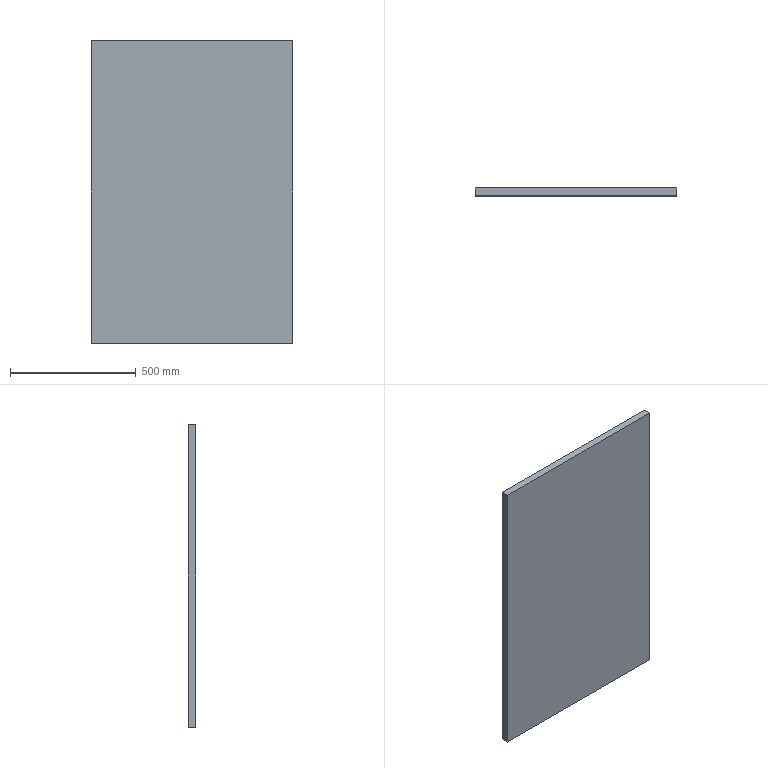Part | 1 solid | 6 faces | box 800 x 30 x 1200 mm | volume 28800000 mm3 | plane 6
STEP:
#1=CARTESIAN_POINT('',(400.,0.,600.));
#2=VERTEX_POINT('',#1);
#3=CARTESIAN_POINT('',(400.,0.,-600.));
#4=VERTEX_POINT('',#3);
#5=CARTESIAN_POINT('',(400.,0.,600.));
#6=DIRECTION('',(0.,0.,-1.));
#7=VECTOR('',#6,1000.);
#8=LINE('',#5,#7);
#9=EDGE_CURVE('',#2,#4,#8,.T.);
#10=ORIENTED_EDGE('',*,*,#9,.T.);
#11=CARTESIAN_POINT('',(400.,30.,-600.));
#12=VERTEX_POINT('',#11);
#13=CARTESIAN_POINT('',(400.,30.,-600.));
#14=DIRECTION('',(0.,-1.,0.));
#15=VECTOR('',#14,1000.);
#16=LINE('',#13,#15);
#17=EDGE_CURVE('',#12,#4,#16,.T.);
#18=ORIENTED_EDGE('',*,*,#17,.F.);
#19=CARTESIAN_POINT('',(400.,30.,600.));
#20=VERTEX_POINT('',#19);
#21=CARTESIAN_POINT('',(400.,30.,600.));
#22=DIRECTION('',(0.,0.,-1.));
#23=VECTOR('',#22,1000.);
#24=LINE('',#21,#23);
#25=EDGE_CURVE('',#20,#12,#24,.T.);
#26=ORIENTED_EDGE('',*,*,#25,.F.);
#27=CARTESIAN_POINT('',(400.,30.,600.));
#28=DIRECTION('',(0.,-1.,0.));
#29=VECTOR('',#28,1000.);
#30=LINE('',#27,#29);
#31=EDGE_CURVE('',#20,#2,#30,.T.);
#32=ORIENTED_EDGE('',*,*,#31,.T.);
#33=EDGE_LOOP('',(#10,#18,#26,#32));
#34=FACE_OUTER_BOUND('',#33,.T.);
#35=CARTESIAN_POINT('',(400.,30.,600.));
#36=DIRECTION('',(-1.,0.,0.));
#37=DIRECTION('',(0.,0.,1.));
#38=AXIS2_PLACEMENT_3D('',#35,#36,#37);
#39=PLANE('',#38);
#40=ADVANCED_FACE('',(#34),#39,.F.);
#41=CARTESIAN_POINT('',(-400.,0.,-600.));
#42=VERTEX_POINT('',#41);
#43=CARTESIAN_POINT('',(-400.,0.,-600.));
#44=DIRECTION('',(-1.,0.,0.));
#45=VECTOR('',#44,1000.);
#46=LINE('',#43,#45);
#47=EDGE_CURVE('',#4,#42,#46,.T.);
#48=ORIENTED_EDGE('',*,*,#47,.T.);
#49=CARTESIAN_POINT('',(-400.,30.,-600.));
#50=VERTEX_POINT('',#49);
#51=CARTESIAN_POINT('',(-400.,30.,-600.));
#52=DIRECTION('',(0.,-1.,0.));
#53=VECTOR('',#52,1000.);
#54=LINE('',#51,#53);
#55=EDGE_CURVE('',#50,#42,#54,.T.);
#56=ORIENTED_EDGE('',*,*,#55,.F.);
#57=CARTESIAN_POINT('',(-400.,30.,-600.));
#58=DIRECTION('',(-1.,0.,0.));
#59=VECTOR('',#58,1000.);
#60=LINE('',#57,#59);
#61=EDGE_CURVE('',#12,#50,#60,.T.);
#62=ORIENTED_EDGE('',*,*,#61,.F.);
#63=ORIENTED_EDGE('',*,*,#17,.T.);
#64=EDGE_LOOP('',(#48,#56,#62,#63));
#65=FACE_OUTER_BOUND('',#64,.T.);
#66=CARTESIAN_POINT('',(-400.,30.,-600.));
#67=DIRECTION('',(0.,0.,1.));
#68=DIRECTION('',(1.,0.,0.));
#69=AXIS2_PLACEMENT_3D('',#66,#67,#68);
#70=PLANE('',#69);
#71=ADVANCED_FACE('',(#65),#70,.F.);
#72=CARTESIAN_POINT('',(-400.,0.,600.));
#73=VERTEX_POINT('',#72);
#74=CARTESIAN_POINT('',(-400.,0.,600.));
#75=DIRECTION('',(0.,0.,1.));
#76=VECTOR('',#75,1000.);
#77=LINE('',#74,#76);
#78=EDGE_CURVE('',#42,#73,#77,.T.);
#79=ORIENTED_EDGE('',*,*,#78,.T.);
#80=CARTESIAN_POINT('',(-400.,30.,600.));
#81=VERTEX_POINT('',#80);
#82=CARTESIAN_POINT('',(-400.,30.,600.));
#83=DIRECTION('',(0.,-1.,0.));
#84=VECTOR('',#83,1000.);
#85=LINE('',#82,#84);
#86=EDGE_CURVE('',#81,#73,#85,.T.);
#87=ORIENTED_EDGE('',*,*,#86,.F.);
#88=CARTESIAN_POINT('',(-400.,30.,600.));
#89=DIRECTION('',(0.,0.,1.));
#90=VECTOR('',#89,1000.);
#91=LINE('',#88,#90);
#92=EDGE_CURVE('',#50,#81,#91,.T.);
#93=ORIENTED_EDGE('',*,*,#92,.F.);
#94=ORIENTED_EDGE('',*,*,#55,.T.);
#95=EDGE_LOOP('',(#79,#87,#93,#94));
#96=FACE_OUTER_BOUND('',#95,.T.);
#97=CARTESIAN_POINT('',(-400.,30.,600.));
#98=DIRECTION('',(1.,0.,0.));
#99=DIRECTION('',(0.,0.,-1.));
#100=AXIS2_PLACEMENT_3D('',#97,#98,#99);
#101=PLANE('',#100);
#102=ADVANCED_FACE('',(#96),#101,.F.);
#103=CARTESIAN_POINT('',(-400.,0.,600.));
#104=DIRECTION('',(1.,0.,0.));
#105=VECTOR('',#104,1000.);
#106=LINE('',#103,#105);
#107=EDGE_CURVE('',#73,#2,#106,.T.);
#108=ORIENTED_EDGE('',*,*,#107,.T.);
#109=ORIENTED_EDGE('',*,*,#31,.F.);
#110=CARTESIAN_POINT('',(-400.,30.,600.));
#111=DIRECTION('',(1.,0.,0.));
#112=VECTOR('',#111,1000.);
#113=LINE('',#110,#112);
#114=EDGE_CURVE('',#81,#20,#113,.T.);
#115=ORIENTED_EDGE('',*,*,#114,.F.);
#116=ORIENTED_EDGE('',*,*,#86,.T.);
#117=EDGE_LOOP('',(#108,#109,#115,#116));
#118=FACE_OUTER_BOUND('',#117,.T.);
#119=CARTESIAN_POINT('',(-400.,30.,600.));
#120=DIRECTION('',(0.,0.,-1.));
#121=DIRECTION('',(-1.,0.,0.));
#122=AXIS2_PLACEMENT_3D('',#119,#120,#121);
#123=PLANE('',#122);
#124=ADVANCED_FACE('',(#118),#123,.F.);
#125=ORIENTED_EDGE('',*,*,#25,.T.);
#126=ORIENTED_EDGE('',*,*,#61,.T.);
#127=ORIENTED_EDGE('',*,*,#92,.T.);
#128=ORIENTED_EDGE('',*,*,#114,.T.);
#129=EDGE_LOOP('',(#125,#126,#127,#128));
#130=FACE_OUTER_BOUND('',#129,.T.);
#131=CARTESIAN_POINT('',(0.,30.,0.));
#132=DIRECTION('',(0.,-1.,0.));
#133=DIRECTION('',(0.,0.,-1.));
#134=AXIS2_PLACEMENT_3D('',#131,#132,#133);
#135=PLANE('',#134);
#136=ADVANCED_FACE('',(#130),#135,.F.);
#137=ORIENTED_EDGE('',*,*,#9,.F.);
#138=ORIENTED_EDGE('',*,*,#107,.F.);
#139=ORIENTED_EDGE('',*,*,#78,.F.);
#140=ORIENTED_EDGE('',*,*,#47,.F.);
#141=EDGE_LOOP('',(#137,#138,#139,#140));
#142=FACE_OUTER_BOUND('',#141,.T.);
#143=CARTESIAN_POINT('',(0.,0.,0.));
#144=DIRECTION('',(0.,-1.,0.));
#145=DIRECTION('',(0.,0.,-1.));
#146=AXIS2_PLACEMENT_3D('',#143,#144,#145);
#147=PLANE('',#146);
#148=ADVANCED_FACE('',(#142),#147,.T.);
#149=CLOSED_SHELL('',(#40,#71,#102,#124,#136,#148));
#150=MANIFOLD_SOLID_BREP('',#149);
#151=CARTESIAN_POINT('',(0.,0.,0.));
#152=DIRECTION('',(0.,0.,1.));
#153=DIRECTION('',(1.,0.,0.));
#154=AXIS2_PLACEMENT_3D('',#151,#152,#153);
#155=(LENGTH_UNIT()NAMED_UNIT(*)SI_UNIT(.MILLI.,.METRE.));
#156=UNCERTAINTY_MEASURE_WITH_UNIT(LENGTH_MEASURE(0.00001),#155,'','');
#157=(NAMED_UNIT(*)PLANE_ANGLE_UNIT()SI_UNIT($,.RADIAN.));
#158=(NAMED_UNIT(*)SI_UNIT($,.STERADIAN.)SOLID_ANGLE_UNIT());
#159=(GEOMETRIC_REPRESENTATION_CONTEXT(3)GLOBAL_UNCERTAINTY_ASSIGNED_CONTEXT((#156))GLOBAL_UNIT_ASSIGNED_CONTEXT((#155,#157,#158))REPRESENTATION_CONTEXT('',''));
#160=ADVANCED_BREP_SHAPE_REPRESENTATION('',(#150,#154),#159);